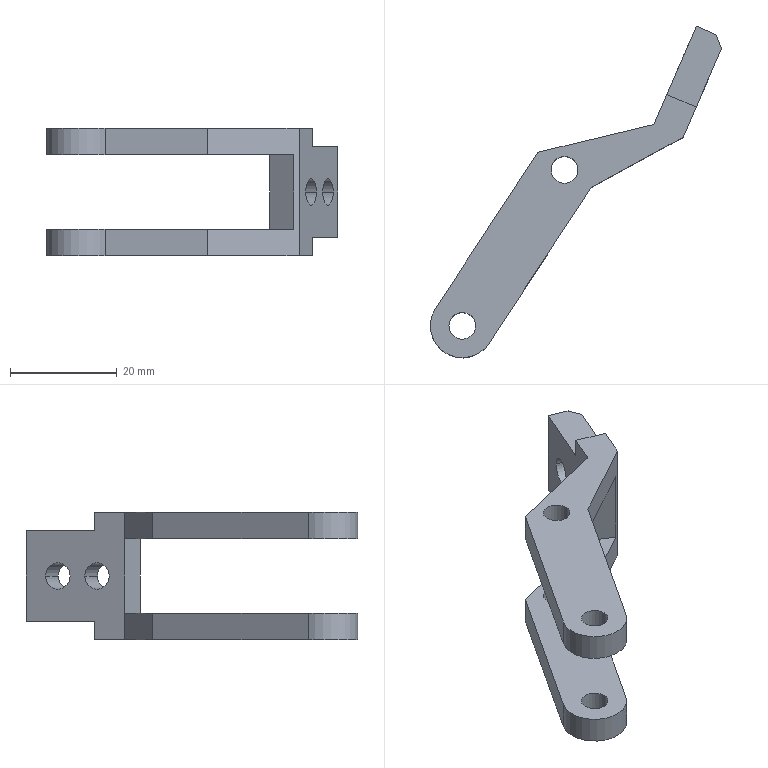Part | STEP file | gripper arm 3_default | 1 solid | 34 faces | box 54.647 x 62.275 x 24 mm | volume 7898 mm3 | plane 20 | cylinder 14 | commonest cylinder face diameters 5 x12 12 x2